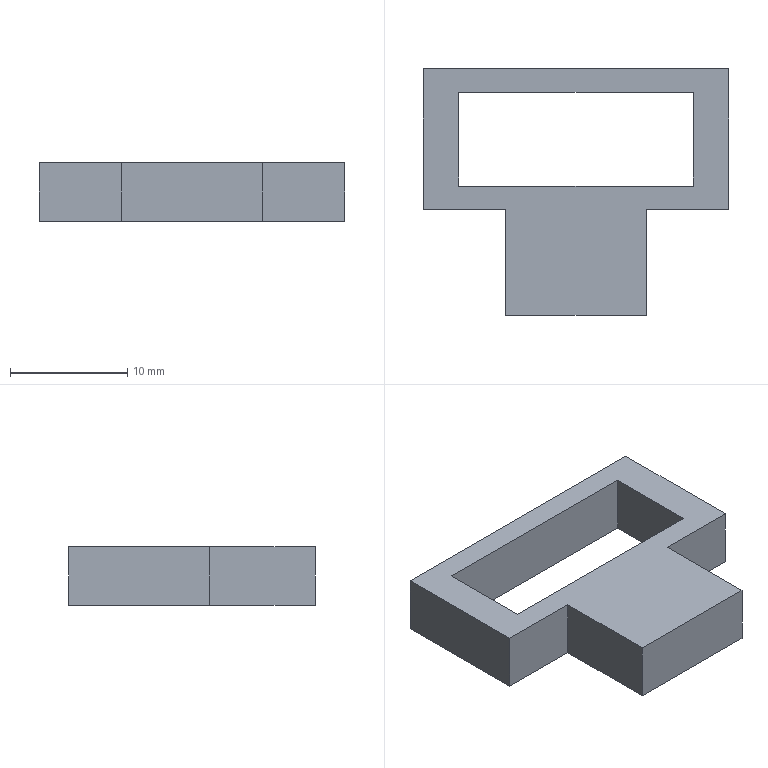Part | SolidWorks | features Extrusion 1, ICE 1 | 1 solid | 14 faces | box 26 x 21 x 5 mm | volume 1300 mm3 | plane 14
STEP:
#1=CARTESIAN_POINT('',(-13.,-6.,-2.5));
#2=VERTEX_POINT('',#1);
#3=CARTESIAN_POINT('',(-6.,-6.,-2.5));
#4=VERTEX_POINT('',#3);
#5=CARTESIAN_POINT('',(-13.,-6.,-2.5));
#6=DIRECTION('',(1.,0.,0.));
#7=VECTOR('',#6,1000.);
#8=LINE('',#5,#7);
#9=EDGE_CURVE('',#2,#4,#8,.T.);
#10=ORIENTED_EDGE('',*,*,#9,.T.);
#11=CARTESIAN_POINT('',(-6.,-6.,2.5));
#12=VERTEX_POINT('',#11);
#13=CARTESIAN_POINT('',(-6.,-6.,-2.5));
#14=DIRECTION('',(0.,0.,1.));
#15=VECTOR('',#14,1000.);
#16=LINE('',#13,#15);
#17=EDGE_CURVE('',#4,#12,#16,.T.);
#18=ORIENTED_EDGE('',*,*,#17,.T.);
#19=CARTESIAN_POINT('',(-13.,-6.,2.5));
#20=VERTEX_POINT('',#19);
#21=CARTESIAN_POINT('',(-13.,-6.,2.5));
#22=DIRECTION('',(1.,0.,0.));
#23=VECTOR('',#22,1000.);
#24=LINE('',#21,#23);
#25=EDGE_CURVE('',#20,#12,#24,.T.);
#26=ORIENTED_EDGE('',*,*,#25,.F.);
#27=CARTESIAN_POINT('',(-13.,-6.,-2.5));
#28=DIRECTION('',(0.,0.,1.));
#29=VECTOR('',#28,1000.);
#30=LINE('',#27,#29);
#31=EDGE_CURVE('',#2,#20,#30,.T.);
#32=ORIENTED_EDGE('',*,*,#31,.F.);
#33=EDGE_LOOP('',(#10,#18,#26,#32));
#34=FACE_OUTER_BOUND('',#33,.T.);
#35=CARTESIAN_POINT('',(-13.,-6.,-2.5));
#36=DIRECTION('',(0.,-1.,0.));
#37=DIRECTION('',(0.,0.,-1.));
#38=AXIS2_PLACEMENT_3D('',#35,#36,#37);
#39=PLANE('',#38);
#40=ADVANCED_FACE('',(#34),#39,.T.);
#41=CARTESIAN_POINT('',(-13.,6.,2.5));
#42=VERTEX_POINT('',#41);
#43=CARTESIAN_POINT('',(-13.,6.,2.5));
#44=DIRECTION('',(0.,-1.,0.));
#45=VECTOR('',#44,1000.);
#46=LINE('',#43,#45);
#47=EDGE_CURVE('',#42,#20,#46,.T.);
#48=ORIENTED_EDGE('',*,*,#47,.F.);
#49=CARTESIAN_POINT('',(-13.,6.,-2.5));
#50=VERTEX_POINT('',#49);
#51=CARTESIAN_POINT('',(-13.,6.,-2.5));
#52=DIRECTION('',(0.,0.,1.));
#53=VECTOR('',#52,1000.);
#54=LINE('',#51,#53);
#55=EDGE_CURVE('',#50,#42,#54,.T.);
#56=ORIENTED_EDGE('',*,*,#55,.F.);
#57=CARTESIAN_POINT('',(-13.,6.,-2.5));
#58=DIRECTION('',(0.,-1.,0.));
#59=VECTOR('',#58,1000.);
#60=LINE('',#57,#59);
#61=EDGE_CURVE('',#50,#2,#60,.T.);
#62=ORIENTED_EDGE('',*,*,#61,.T.);
#63=ORIENTED_EDGE('',*,*,#31,.T.);
#64=EDGE_LOOP('',(#48,#56,#62,#63));
#65=FACE_OUTER_BOUND('',#64,.T.);
#66=CARTESIAN_POINT('',(-13.,6.,-2.5));
#67=DIRECTION('',(-1.,0.,0.));
#68=DIRECTION('',(0.,0.,1.));
#69=AXIS2_PLACEMENT_3D('',#66,#67,#68);
#70=PLANE('',#69);
#71=ADVANCED_FACE('',(#65),#70,.T.);
#72=CARTESIAN_POINT('',(13.,6.,2.5));
#73=VERTEX_POINT('',#72);
#74=CARTESIAN_POINT('',(13.,6.,2.5));
#75=DIRECTION('',(-1.,0.,0.));
#76=VECTOR('',#75,1000.);
#77=LINE('',#74,#76);
#78=EDGE_CURVE('',#73,#42,#77,.T.);
#79=ORIENTED_EDGE('',*,*,#78,.F.);
#80=CARTESIAN_POINT('',(13.,6.,-2.5));
#81=VERTEX_POINT('',#80);
#82=CARTESIAN_POINT('',(13.,6.,-2.5));
#83=DIRECTION('',(0.,0.,1.));
#84=VECTOR('',#83,1000.);
#85=LINE('',#82,#84);
#86=EDGE_CURVE('',#81,#73,#85,.T.);
#87=ORIENTED_EDGE('',*,*,#86,.F.);
#88=CARTESIAN_POINT('',(13.,6.,-2.5));
#89=DIRECTION('',(-1.,0.,0.));
#90=VECTOR('',#89,1000.);
#91=LINE('',#88,#90);
#92=EDGE_CURVE('',#81,#50,#91,.T.);
#93=ORIENTED_EDGE('',*,*,#92,.T.);
#94=ORIENTED_EDGE('',*,*,#55,.T.);
#95=EDGE_LOOP('',(#79,#87,#93,#94));
#96=FACE_OUTER_BOUND('',#95,.T.);
#97=CARTESIAN_POINT('',(13.,6.,-2.5));
#98=DIRECTION('',(0.,1.,0.));
#99=DIRECTION('',(0.,0.,1.));
#100=AXIS2_PLACEMENT_3D('',#97,#98,#99);
#101=PLANE('',#100);
#102=ADVANCED_FACE('',(#96),#101,.T.);
#103=CARTESIAN_POINT('',(13.,-6.,2.5));
#104=VERTEX_POINT('',#103);
#105=CARTESIAN_POINT('',(13.,-6.,2.5));
#106=DIRECTION('',(0.,1.,0.));
#107=VECTOR('',#106,1000.);
#108=LINE('',#105,#107);
#109=EDGE_CURVE('',#104,#73,#108,.T.);
#110=ORIENTED_EDGE('',*,*,#109,.F.);
#111=CARTESIAN_POINT('',(13.,-6.,-2.5));
#112=VERTEX_POINT('',#111);
#113=CARTESIAN_POINT('',(13.,-6.,-2.5));
#114=DIRECTION('',(0.,0.,1.));
#115=VECTOR('',#114,1000.);
#116=LINE('',#113,#115);
#117=EDGE_CURVE('',#112,#104,#116,.T.);
#118=ORIENTED_EDGE('',*,*,#117,.F.);
#119=CARTESIAN_POINT('',(13.,-6.,-2.5));
#120=DIRECTION('',(0.,1.,0.));
#121=VECTOR('',#120,1000.);
#122=LINE('',#119,#121);
#123=EDGE_CURVE('',#112,#81,#122,.T.);
#124=ORIENTED_EDGE('',*,*,#123,.T.);
#125=ORIENTED_EDGE('',*,*,#86,.T.);
#126=EDGE_LOOP('',(#110,#118,#124,#125));
#127=FACE_OUTER_BOUND('',#126,.T.);
#128=CARTESIAN_POINT('',(13.,-6.,-2.5));
#129=DIRECTION('',(1.,0.,0.));
#130=DIRECTION('',(0.,0.,-1.));
#131=AXIS2_PLACEMENT_3D('',#128,#129,#130);
#132=PLANE('',#131);
#133=ADVANCED_FACE('',(#127),#132,.T.);
#134=CARTESIAN_POINT('',(6.,-6.,-2.5));
#135=VERTEX_POINT('',#134);
#136=CARTESIAN_POINT('',(6.,-6.,2.5));
#137=VERTEX_POINT('',#136);
#138=CARTESIAN_POINT('',(6.,-6.,-2.5));
#139=DIRECTION('',(0.,0.,1.));
#140=VECTOR('',#139,1000.);
#141=LINE('',#138,#140);
#142=EDGE_CURVE('',#135,#137,#141,.T.);
#143=ORIENTED_EDGE('',*,*,#142,.F.);
#144=CARTESIAN_POINT('',(-13.,-6.,-2.5));
#145=DIRECTION('',(1.,0.,0.));
#146=VECTOR('',#145,1000.);
#147=LINE('',#144,#146);
#148=EDGE_CURVE('',#135,#112,#147,.T.);
#149=ORIENTED_EDGE('',*,*,#148,.T.);
#150=ORIENTED_EDGE('',*,*,#117,.T.);
#151=CARTESIAN_POINT('',(-13.,-6.,2.5));
#152=DIRECTION('',(1.,0.,0.));
#153=VECTOR('',#152,1000.);
#154=LINE('',#151,#153);
#155=EDGE_CURVE('',#137,#104,#154,.T.);
#156=ORIENTED_EDGE('',*,*,#155,.F.);
#157=EDGE_LOOP('',(#143,#149,#150,#156));
#158=FACE_OUTER_BOUND('',#157,.T.);
#159=CARTESIAN_POINT('',(-13.,-6.,-2.5));
#160=DIRECTION('',(0.,-1.,0.));
#161=DIRECTION('',(0.,0.,-1.));
#162=AXIS2_PLACEMENT_3D('',#159,#160,#161);
#163=PLANE('',#162);
#164=ADVANCED_FACE('',(#158),#163,.T.);
#165=CARTESIAN_POINT('',(10.,4.,-2.5));
#166=VERTEX_POINT('',#165);
#167=CARTESIAN_POINT('',(-10.,4.,-2.5));
#168=VERTEX_POINT('',#167);
#169=CARTESIAN_POINT('',(10.,4.,-2.5));
#170=DIRECTION('',(-1.,0.,0.));
#171=VECTOR('',#170,1000.);
#172=LINE('',#169,#171);
#173=EDGE_CURVE('',#166,#168,#172,.T.);
#174=ORIENTED_EDGE('',*,*,#173,.T.);
#175=CARTESIAN_POINT('',(-10.,-4.,-2.5));
#176=VERTEX_POINT('',#175);
#177=CARTESIAN_POINT('',(-10.,4.,-2.5));
#178=DIRECTION('',(0.,-1.,0.));
#179=VECTOR('',#178,1000.);
#180=LINE('',#177,#179);
#181=EDGE_CURVE('',#168,#176,#180,.T.);
#182=ORIENTED_EDGE('',*,*,#181,.T.);
#183=CARTESIAN_POINT('',(10.,-4.,-2.5));
#184=VERTEX_POINT('',#183);
#185=CARTESIAN_POINT('',(-10.,-4.,-2.5));
#186=DIRECTION('',(1.,0.,0.));
#187=VECTOR('',#186,1000.);
#188=LINE('',#185,#187);
#189=EDGE_CURVE('',#176,#184,#188,.T.);
#190=ORIENTED_EDGE('',*,*,#189,.T.);
#191=CARTESIAN_POINT('',(10.,-4.,-2.5));
#192=DIRECTION('',(0.,1.,0.));
#193=VECTOR('',#192,1000.);
#194=LINE('',#191,#193);
#195=EDGE_CURVE('',#184,#166,#194,.T.);
#196=ORIENTED_EDGE('',*,*,#195,.T.);
#197=EDGE_LOOP('',(#174,#182,#190,#196));
#198=FACE_BOUND('',#197,.T.);
#199=ORIENTED_EDGE('',*,*,#61,.F.);
#200=ORIENTED_EDGE('',*,*,#92,.F.);
#201=ORIENTED_EDGE('',*,*,#123,.F.);
#202=ORIENTED_EDGE('',*,*,#148,.F.);
#203=CARTESIAN_POINT('',(6.,-15.,-2.5));
#204=VERTEX_POINT('',#203);
#205=CARTESIAN_POINT('',(6.,-15.,-2.5));
#206=DIRECTION('',(0.,1.,0.));
#207=VECTOR('',#206,1000.);
#208=LINE('',#205,#207);
#209=EDGE_CURVE('',#204,#135,#208,.T.);
#210=ORIENTED_EDGE('',*,*,#209,.F.);
#211=CARTESIAN_POINT('',(-6.,-15.,-2.5));
#212=VERTEX_POINT('',#211);
#213=CARTESIAN_POINT('',(-6.,-15.,-2.5));
#214=DIRECTION('',(1.,0.,0.));
#215=VECTOR('',#214,1000.);
#216=LINE('',#213,#215);
#217=EDGE_CURVE('',#212,#204,#216,.T.);
#218=ORIENTED_EDGE('',*,*,#217,.F.);
#219=CARTESIAN_POINT('',(-6.,-6.,-2.5));
#220=DIRECTION('',(0.,-1.,0.));
#221=VECTOR('',#220,1000.);
#222=LINE('',#219,#221);
#223=EDGE_CURVE('',#4,#212,#222,.T.);
#224=ORIENTED_EDGE('',*,*,#223,.F.);
#225=ORIENTED_EDGE('',*,*,#9,.F.);
#226=EDGE_LOOP('',(#199,#200,#201,#202,#210,#218,#224,#225));
#227=FACE_OUTER_BOUND('',#226,.T.);
#228=CARTESIAN_POINT('',(0.,0.,-2.5));
#229=DIRECTION('',(0.,0.,1.));
#230=DIRECTION('',(1.,0.,0.));
#231=AXIS2_PLACEMENT_3D('',#228,#229,#230);
#232=PLANE('',#231);
#233=ADVANCED_FACE('',(#198,#227),#232,.F.);
#234=CARTESIAN_POINT('',(-10.,4.,2.5));
#235=VERTEX_POINT('',#234);
#236=CARTESIAN_POINT('',(-10.,-4.,2.5));
#237=VERTEX_POINT('',#236);
#238=CARTESIAN_POINT('',(-10.,4.,2.5));
#239=DIRECTION('',(0.,-1.,0.));
#240=VECTOR('',#239,1000.);
#241=LINE('',#238,#240);
#242=EDGE_CURVE('',#235,#237,#241,.T.);
#243=ORIENTED_EDGE('',*,*,#242,.F.);
#244=CARTESIAN_POINT('',(10.,4.,2.5));
#245=VERTEX_POINT('',#244);
#246=CARTESIAN_POINT('',(10.,4.,2.5));
#247=DIRECTION('',(-1.,0.,0.));
#248=VECTOR('',#247,1000.);
#249=LINE('',#246,#248);
#250=EDGE_CURVE('',#245,#235,#249,.T.);
#251=ORIENTED_EDGE('',*,*,#250,.F.);
#252=CARTESIAN_POINT('',(10.,-4.,2.5));
#253=VERTEX_POINT('',#252);
#254=CARTESIAN_POINT('',(10.,-4.,2.5));
#255=DIRECTION('',(0.,1.,0.));
#256=VECTOR('',#255,1000.);
#257=LINE('',#254,#256);
#258=EDGE_CURVE('',#253,#245,#257,.T.);
#259=ORIENTED_EDGE('',*,*,#258,.F.);
#260=CARTESIAN_POINT('',(-10.,-4.,2.5));
#261=DIRECTION('',(1.,0.,0.));
#262=VECTOR('',#261,1000.);
#263=LINE('',#260,#262);
#264=EDGE_CURVE('',#237,#253,#263,.T.);
#265=ORIENTED_EDGE('',*,*,#264,.F.);
#266=EDGE_LOOP('',(#243,#251,#259,#265));
#267=FACE_BOUND('',#266,.T.);
#268=ORIENTED_EDGE('',*,*,#47,.T.);
#269=ORIENTED_EDGE('',*,*,#25,.T.);
#270=CARTESIAN_POINT('',(-6.,-15.,2.5));
#271=VERTEX_POINT('',#270);
#272=CARTESIAN_POINT('',(-6.,-6.,2.5));
#273=DIRECTION('',(0.,-1.,0.));
#274=VECTOR('',#273,1000.);
#275=LINE('',#272,#274);
#276=EDGE_CURVE('',#12,#271,#275,.T.);
#277=ORIENTED_EDGE('',*,*,#276,.T.);
#278=CARTESIAN_POINT('',(6.,-15.,2.5));
#279=VERTEX_POINT('',#278);
#280=CARTESIAN_POINT('',(-6.,-15.,2.5));
#281=DIRECTION('',(1.,0.,0.));
#282=VECTOR('',#281,1000.);
#283=LINE('',#280,#282);
#284=EDGE_CURVE('',#271,#279,#283,.T.);
#285=ORIENTED_EDGE('',*,*,#284,.T.);
#286=CARTESIAN_POINT('',(6.,-15.,2.5));
#287=DIRECTION('',(0.,1.,0.));
#288=VECTOR('',#287,1000.);
#289=LINE('',#286,#288);
#290=EDGE_CURVE('',#279,#137,#289,.T.);
#291=ORIENTED_EDGE('',*,*,#290,.T.);
#292=ORIENTED_EDGE('',*,*,#155,.T.);
#293=ORIENTED_EDGE('',*,*,#109,.T.);
#294=ORIENTED_EDGE('',*,*,#78,.T.);
#295=EDGE_LOOP('',(#268,#269,#277,#285,#291,#292,#293,#294));
#296=FACE_OUTER_BOUND('',#295,.T.);
#297=CARTESIAN_POINT('',(0.,0.,2.5));
#298=DIRECTION('',(0.,0.,1.));
#299=DIRECTION('',(1.,0.,0.));
#300=AXIS2_PLACEMENT_3D('',#297,#298,#299);
#301=PLANE('',#300);
#302=ADVANCED_FACE('',(#267,#296),#301,.T.);
#303=ORIENTED_EDGE('',*,*,#242,.T.);
#304=CARTESIAN_POINT('',(-10.,-4.,-2.5));
#305=DIRECTION('',(0.,0.,1.));
#306=VECTOR('',#305,1000.);
#307=LINE('',#304,#306);
#308=EDGE_CURVE('',#176,#237,#307,.T.);
#309=ORIENTED_EDGE('',*,*,#308,.F.);
#310=ORIENTED_EDGE('',*,*,#181,.F.);
#311=CARTESIAN_POINT('',(-10.,4.,-2.5));
#312=DIRECTION('',(0.,0.,1.));
#313=VECTOR('',#312,1000.);
#314=LINE('',#311,#313);
#315=EDGE_CURVE('',#168,#235,#314,.T.);
#316=ORIENTED_EDGE('',*,*,#315,.T.);
#317=EDGE_LOOP('',(#303,#309,#310,#316));
#318=FACE_OUTER_BOUND('',#317,.T.);
#319=CARTESIAN_POINT('',(-10.,4.,-2.5));
#320=DIRECTION('',(-1.,0.,0.));
#321=DIRECTION('',(0.,0.,1.));
#322=AXIS2_PLACEMENT_3D('',#319,#320,#321);
#323=PLANE('',#322);
#324=ADVANCED_FACE('',(#318),#323,.F.);
#325=ORIENTED_EDGE('',*,*,#250,.T.);
#326=ORIENTED_EDGE('',*,*,#315,.F.);
#327=ORIENTED_EDGE('',*,*,#173,.F.);
#328=CARTESIAN_POINT('',(10.,4.,-2.5));
#329=DIRECTION('',(0.,0.,1.));
#330=VECTOR('',#329,1000.);
#331=LINE('',#328,#330);
#332=EDGE_CURVE('',#166,#245,#331,.T.);
#333=ORIENTED_EDGE('',*,*,#332,.T.);
#334=EDGE_LOOP('',(#325,#326,#327,#333));
#335=FACE_OUTER_BOUND('',#334,.T.);
#336=CARTESIAN_POINT('',(10.,4.,-2.5));
#337=DIRECTION('',(0.,1.,0.));
#338=DIRECTION('',(0.,0.,1.));
#339=AXIS2_PLACEMENT_3D('',#336,#337,#338);
#340=PLANE('',#339);
#341=ADVANCED_FACE('',(#335),#340,.F.);
#342=ORIENTED_EDGE('',*,*,#258,.T.);
#343=ORIENTED_EDGE('',*,*,#332,.F.);
#344=ORIENTED_EDGE('',*,*,#195,.F.);
#345=CARTESIAN_POINT('',(10.,-4.,-2.5));
#346=DIRECTION('',(0.,0.,1.));
#347=VECTOR('',#346,1000.);
#348=LINE('',#345,#347);
#349=EDGE_CURVE('',#184,#253,#348,.T.);
#350=ORIENTED_EDGE('',*,*,#349,.T.);
#351=EDGE_LOOP('',(#342,#343,#344,#350));
#352=FACE_OUTER_BOUND('',#351,.T.);
#353=CARTESIAN_POINT('',(10.,-4.,-2.5));
#354=DIRECTION('',(1.,0.,0.));
#355=DIRECTION('',(0.,0.,-1.));
#356=AXIS2_PLACEMENT_3D('',#353,#354,#355);
#357=PLANE('',#356);
#358=ADVANCED_FACE('',(#352),#357,.F.);
#359=ORIENTED_EDGE('',*,*,#264,.T.);
#360=ORIENTED_EDGE('',*,*,#349,.F.);
#361=ORIENTED_EDGE('',*,*,#189,.F.);
#362=ORIENTED_EDGE('',*,*,#308,.T.);
#363=EDGE_LOOP('',(#359,#360,#361,#362));
#364=FACE_OUTER_BOUND('',#363,.T.);
#365=CARTESIAN_POINT('',(-10.,-4.,-2.5));
#366=DIRECTION('',(0.,-1.,0.));
#367=DIRECTION('',(0.,0.,-1.));
#368=AXIS2_PLACEMENT_3D('',#365,#366,#367);
#369=PLANE('',#368);
#370=ADVANCED_FACE('',(#364),#369,.F.);
#371=ORIENTED_EDGE('',*,*,#276,.F.);
#372=ORIENTED_EDGE('',*,*,#17,.F.);
#373=ORIENTED_EDGE('',*,*,#223,.T.);
#374=CARTESIAN_POINT('',(-6.,-15.,-2.5));
#375=DIRECTION('',(0.,0.,1.));
#376=VECTOR('',#375,1000.);
#377=LINE('',#374,#376);
#378=EDGE_CURVE('',#212,#271,#377,.T.);
#379=ORIENTED_EDGE('',*,*,#378,.T.);
#380=EDGE_LOOP('',(#371,#372,#373,#379));
#381=FACE_OUTER_BOUND('',#380,.T.);
#382=CARTESIAN_POINT('',(-6.,-6.,-2.5));
#383=DIRECTION('',(-1.,0.,0.));
#384=DIRECTION('',(0.,0.,1.));
#385=AXIS2_PLACEMENT_3D('',#382,#383,#384);
#386=PLANE('',#385);
#387=ADVANCED_FACE('',(#381),#386,.T.);
#388=ORIENTED_EDGE('',*,*,#290,.F.);
#389=CARTESIAN_POINT('',(6.,-15.,-2.5));
#390=DIRECTION('',(0.,0.,1.));
#391=VECTOR('',#390,1000.);
#392=LINE('',#389,#391);
#393=EDGE_CURVE('',#204,#279,#392,.T.);
#394=ORIENTED_EDGE('',*,*,#393,.F.);
#395=ORIENTED_EDGE('',*,*,#209,.T.);
#396=ORIENTED_EDGE('',*,*,#142,.T.);
#397=EDGE_LOOP('',(#388,#394,#395,#396));
#398=FACE_OUTER_BOUND('',#397,.T.);
#399=CARTESIAN_POINT('',(6.,-15.,-2.5));
#400=DIRECTION('',(1.,0.,0.));
#401=DIRECTION('',(0.,0.,-1.));
#402=AXIS2_PLACEMENT_3D('',#399,#400,#401);
#403=PLANE('',#402);
#404=ADVANCED_FACE('',(#398),#403,.T.);
#405=ORIENTED_EDGE('',*,*,#284,.F.);
#406=ORIENTED_EDGE('',*,*,#378,.F.);
#407=ORIENTED_EDGE('',*,*,#217,.T.);
#408=ORIENTED_EDGE('',*,*,#393,.T.);
#409=EDGE_LOOP('',(#405,#406,#407,#408));
#410=FACE_OUTER_BOUND('',#409,.T.);
#411=CARTESIAN_POINT('',(-6.,-15.,-2.5));
#412=DIRECTION('',(0.,-1.,0.));
#413=DIRECTION('',(0.,0.,-1.));
#414=AXIS2_PLACEMENT_3D('',#411,#412,#413);
#415=PLANE('',#414);
#416=ADVANCED_FACE('',(#410),#415,.T.);
#417=CLOSED_SHELL('',(#40,#71,#102,#133,#164,#233,#302,#324,#341,#358,#370,#387,#404,#416));
#418=MANIFOLD_SOLID_BREP('',#417);
#419=CARTESIAN_POINT('',(0.,0.,0.));
#420=DIRECTION('',(0.,0.,1.));
#421=DIRECTION('',(1.,0.,0.));
#422=AXIS2_PLACEMENT_3D('',#419,#420,#421);
#423=(LENGTH_UNIT()NAMED_UNIT(*)SI_UNIT(.MILLI.,.METRE.));
#424=UNCERTAINTY_MEASURE_WITH_UNIT(LENGTH_MEASURE(0.00001),#423,'','');
#425=(NAMED_UNIT(*)PLANE_ANGLE_UNIT()SI_UNIT($,.RADIAN.));
#426=(NAMED_UNIT(*)SI_UNIT($,.STERADIAN.)SOLID_ANGLE_UNIT());
#427=(GEOMETRIC_REPRESENTATION_CONTEXT(3)GLOBAL_UNCERTAINTY_ASSIGNED_CONTEXT((#424))GLOBAL_UNIT_ASSIGNED_CONTEXT((#423,#425,#426))REPRESENTATION_CONTEXT('',''));
#428=ADVANCED_BREP_SHAPE_REPRESENTATION('',(#418,#422),#427);